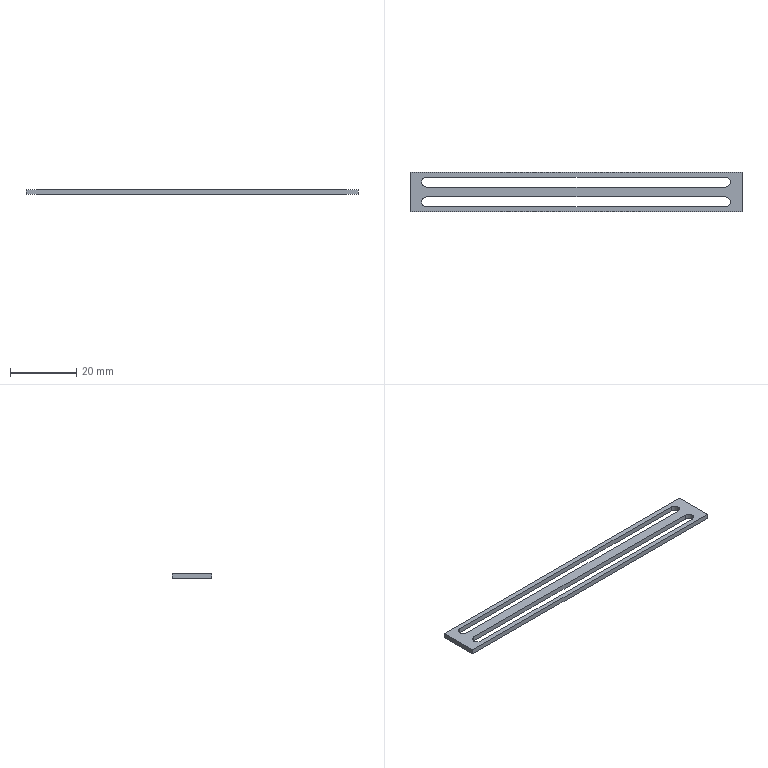Part | SolidWorks | features Extrusion 1 | 1 solid | 16 faces | box 100 x 12 x 1.5 mm | volume 968.794 mm3 | plane 10 | cylinder 6 | commonest cylinder face diameters 3 x6
STEP:
#1=CARTESIAN_POINT('',(-45.,-1.5,1.5));
#2=VERTEX_POINT('',#1);
#3=CARTESIAN_POINT('',(-46.5,-3.,1.5));
#4=VERTEX_POINT('',#3);
#5=CARTESIAN_POINT('',(-45.,-3.,1.5));
#6=DIRECTION('',(0.,0.,1.));
#7=DIRECTION('',(-1.,0.,0.));
#8=AXIS2_PLACEMENT_3D('',#5,#6,#7);
#9=CIRCLE('',#8,1.5);
#10=EDGE_CURVE('',#2,#4,#9,.T.);
#11=ORIENTED_EDGE('',*,*,#10,.T.);
#12=CARTESIAN_POINT('',(-46.5,-3.,0.));
#13=VERTEX_POINT('',#12);
#14=CARTESIAN_POINT('',(-46.5,-3.,1.5));
#15=DIRECTION('',(0.,0.,-1.));
#16=VECTOR('',#15,1000.);
#17=LINE('',#14,#16);
#18=EDGE_CURVE('',#4,#13,#17,.T.);
#19=ORIENTED_EDGE('',*,*,#18,.T.);
#20=CARTESIAN_POINT('',(-45.,-1.5,0.));
#21=VERTEX_POINT('',#20);
#22=CARTESIAN_POINT('',(-45.,-3.,0.));
#23=DIRECTION('',(0.,0.,1.));
#24=DIRECTION('',(-1.,0.,0.));
#25=AXIS2_PLACEMENT_3D('',#22,#23,#24);
#26=CIRCLE('',#25,1.5);
#27=EDGE_CURVE('',#21,#13,#26,.T.);
#28=ORIENTED_EDGE('',*,*,#27,.F.);
#29=CARTESIAN_POINT('',(-45.,-1.5,1.5));
#30=DIRECTION('',(0.,0.,-1.));
#31=VECTOR('',#30,1000.);
#32=LINE('',#29,#31);
#33=EDGE_CURVE('',#2,#21,#32,.T.);
#34=ORIENTED_EDGE('',*,*,#33,.F.);
#35=EDGE_LOOP('',(#11,#19,#28,#34));
#36=FACE_OUTER_BOUND('',#35,.T.);
#37=CARTESIAN_POINT('',(-45.,-3.,1.5));
#38=DIRECTION('',(0.,0.,-1.));
#39=DIRECTION('',(-1.,0.,0.));
#40=AXIS2_PLACEMENT_3D('',#37,#38,#39);
#41=CYLINDRICAL_SURFACE('',#40,1.5);
#42=ADVANCED_FACE('',(#36),#41,.F.);
#43=CARTESIAN_POINT('',(-45.,4.5,1.5));
#44=VERTEX_POINT('',#43);
#45=CARTESIAN_POINT('',(-46.5,3.,1.5));
#46=VERTEX_POINT('',#45);
#47=CARTESIAN_POINT('',(-45.,3.,1.5));
#48=DIRECTION('',(0.,0.,1.));
#49=DIRECTION('',(1.,0.,0.));
#50=AXIS2_PLACEMENT_3D('',#47,#48,#49);
#51=CIRCLE('',#50,1.5);
#52=EDGE_CURVE('',#44,#46,#51,.T.);
#53=ORIENTED_EDGE('',*,*,#52,.T.);
#54=CARTESIAN_POINT('',(-46.5,3.,0.));
#55=VERTEX_POINT('',#54);
#56=CARTESIAN_POINT('',(-46.5,3.,1.5));
#57=DIRECTION('',(0.,0.,-1.));
#58=VECTOR('',#57,1000.);
#59=LINE('',#56,#58);
#60=EDGE_CURVE('',#46,#55,#59,.T.);
#61=ORIENTED_EDGE('',*,*,#60,.T.);
#62=CARTESIAN_POINT('',(-45.,4.5,0.));
#63=VERTEX_POINT('',#62);
#64=CARTESIAN_POINT('',(-45.,3.,0.));
#65=DIRECTION('',(0.,0.,1.));
#66=DIRECTION('',(1.,0.,0.));
#67=AXIS2_PLACEMENT_3D('',#64,#65,#66);
#68=CIRCLE('',#67,1.5);
#69=EDGE_CURVE('',#63,#55,#68,.T.);
#70=ORIENTED_EDGE('',*,*,#69,.F.);
#71=CARTESIAN_POINT('',(-45.,4.5,1.5));
#72=DIRECTION('',(0.,0.,-1.));
#73=VECTOR('',#72,1000.);
#74=LINE('',#71,#73);
#75=EDGE_CURVE('',#44,#63,#74,.T.);
#76=ORIENTED_EDGE('',*,*,#75,.F.);
#77=EDGE_LOOP('',(#53,#61,#70,#76));
#78=FACE_OUTER_BOUND('',#77,.T.);
#79=CARTESIAN_POINT('',(-45.,3.,1.5));
#80=DIRECTION('',(0.,0.,-1.));
#81=DIRECTION('',(-1.,0.,0.));
#82=AXIS2_PLACEMENT_3D('',#79,#80,#81);
#83=CYLINDRICAL_SURFACE('',#82,1.5);
#84=ADVANCED_FACE('',(#78),#83,.F.);
#85=ORIENTED_EDGE('',*,*,#52,.F.);
#86=CARTESIAN_POINT('',(45.,4.5,1.5));
#87=VERTEX_POINT('',#86);
#88=CARTESIAN_POINT('',(-45.,4.5,1.5));
#89=DIRECTION('',(-1.,0.,0.));
#90=VECTOR('',#89,1000.);
#91=LINE('',#88,#90);
#92=EDGE_CURVE('',#87,#44,#91,.T.);
#93=ORIENTED_EDGE('',*,*,#92,.F.);
#94=CARTESIAN_POINT('',(45.,1.5,1.5));
#95=VERTEX_POINT('',#94);
#96=CARTESIAN_POINT('',(45.,3.,1.5));
#97=DIRECTION('',(0.,0.,1.));
#98=DIRECTION('',(1.,0.,0.));
#99=AXIS2_PLACEMENT_3D('',#96,#97,#98);
#100=CIRCLE('',#99,1.5);
#101=EDGE_CURVE('',#95,#87,#100,.T.);
#102=ORIENTED_EDGE('',*,*,#101,.F.);
#103=CARTESIAN_POINT('',(-45.,1.5,1.5));
#104=VERTEX_POINT('',#103);
#105=CARTESIAN_POINT('',(-45.,1.5,1.5));
#106=DIRECTION('',(1.,0.,0.));
#107=VECTOR('',#106,1000.);
#108=LINE('',#105,#107);
#109=EDGE_CURVE('',#104,#95,#108,.T.);
#110=ORIENTED_EDGE('',*,*,#109,.F.);
#111=CARTESIAN_POINT('',(-45.,3.,1.5));
#112=DIRECTION('',(0.,0.,1.));
#113=DIRECTION('',(1.,0.,0.));
#114=AXIS2_PLACEMENT_3D('',#111,#112,#113);
#115=CIRCLE('',#114,1.5);
#116=EDGE_CURVE('',#46,#104,#115,.T.);
#117=ORIENTED_EDGE('',*,*,#116,.F.);
#118=EDGE_LOOP('',(#85,#93,#102,#110,#117));
#119=FACE_BOUND('',#118,.T.);
#120=CARTESIAN_POINT('',(-50.,6.,1.5));
#121=VERTEX_POINT('',#120);
#122=CARTESIAN_POINT('',(-50.,-6.,1.5));
#123=VERTEX_POINT('',#122);
#124=CARTESIAN_POINT('',(-50.,6.,1.5));
#125=DIRECTION('',(0.,-1.,0.));
#126=VECTOR('',#125,1000.);
#127=LINE('',#124,#126);
#128=EDGE_CURVE('',#121,#123,#127,.T.);
#129=ORIENTED_EDGE('',*,*,#128,.T.);
#130=CARTESIAN_POINT('',(50.,-6.,1.5));
#131=VERTEX_POINT('',#130);
#132=CARTESIAN_POINT('',(50.,-6.,1.5));
#133=DIRECTION('',(1.,0.,0.));
#134=VECTOR('',#133,1000.);
#135=LINE('',#132,#134);
#136=EDGE_CURVE('',#123,#131,#135,.T.);
#137=ORIENTED_EDGE('',*,*,#136,.T.);
#138=CARTESIAN_POINT('',(50.,6.,1.5));
#139=VERTEX_POINT('',#138);
#140=CARTESIAN_POINT('',(50.,6.,1.5));
#141=DIRECTION('',(0.,1.,0.));
#142=VECTOR('',#141,1000.);
#143=LINE('',#140,#142);
#144=EDGE_CURVE('',#131,#139,#143,.T.);
#145=ORIENTED_EDGE('',*,*,#144,.T.);
#146=CARTESIAN_POINT('',(50.,6.,1.5));
#147=DIRECTION('',(-1.,0.,0.));
#148=VECTOR('',#147,1000.);
#149=LINE('',#146,#148);
#150=EDGE_CURVE('',#139,#121,#149,.T.);
#151=ORIENTED_EDGE('',*,*,#150,.T.);
#152=EDGE_LOOP('',(#129,#137,#145,#151));
#153=FACE_OUTER_BOUND('',#152,.T.);
#154=ORIENTED_EDGE('',*,*,#10,.F.);
#155=CARTESIAN_POINT('',(45.,-1.5,1.5));
#156=VERTEX_POINT('',#155);
#157=CARTESIAN_POINT('',(-45.,-1.5,1.5));
#158=DIRECTION('',(-1.,0.,0.));
#159=VECTOR('',#158,1000.);
#160=LINE('',#157,#159);
#161=EDGE_CURVE('',#156,#2,#160,.T.);
#162=ORIENTED_EDGE('',*,*,#161,.F.);
#163=CARTESIAN_POINT('',(45.,-4.5,1.5));
#164=VERTEX_POINT('',#163);
#165=CARTESIAN_POINT('',(45.,-3.,1.5));
#166=DIRECTION('',(0.,0.,1.));
#167=DIRECTION('',(-1.,0.,0.));
#168=AXIS2_PLACEMENT_3D('',#165,#166,#167);
#169=CIRCLE('',#168,1.5);
#170=EDGE_CURVE('',#164,#156,#169,.T.);
#171=ORIENTED_EDGE('',*,*,#170,.F.);
#172=CARTESIAN_POINT('',(-45.,-4.5,1.5));
#173=VERTEX_POINT('',#172);
#174=CARTESIAN_POINT('',(-45.,-4.5,1.5));
#175=DIRECTION('',(1.,0.,0.));
#176=VECTOR('',#175,1000.);
#177=LINE('',#174,#176);
#178=EDGE_CURVE('',#173,#164,#177,.T.);
#179=ORIENTED_EDGE('',*,*,#178,.F.);
#180=CARTESIAN_POINT('',(-45.,-3.,1.5));
#181=DIRECTION('',(0.,0.,1.));
#182=DIRECTION('',(-1.,0.,0.));
#183=AXIS2_PLACEMENT_3D('',#180,#181,#182);
#184=CIRCLE('',#183,1.5);
#185=EDGE_CURVE('',#4,#173,#184,.T.);
#186=ORIENTED_EDGE('',*,*,#185,.F.);
#187=EDGE_LOOP('',(#154,#162,#171,#179,#186));
#188=FACE_BOUND('',#187,.T.);
#189=CARTESIAN_POINT('',(0.,0.,1.5));
#190=DIRECTION('',(0.,0.,-1.));
#191=DIRECTION('',(-1.,0.,0.));
#192=AXIS2_PLACEMENT_3D('',#189,#190,#191);
#193=PLANE('',#192);
#194=ADVANCED_FACE('',(#119,#153,#188),#193,.F.);
#195=CARTESIAN_POINT('',(45.,4.5,0.));
#196=VERTEX_POINT('',#195);
#197=CARTESIAN_POINT('',(-45.,4.5,0.));
#198=DIRECTION('',(-1.,0.,0.));
#199=VECTOR('',#198,1000.);
#200=LINE('',#197,#199);
#201=EDGE_CURVE('',#196,#63,#200,.T.);
#202=ORIENTED_EDGE('',*,*,#201,.T.);
#203=ORIENTED_EDGE('',*,*,#69,.T.);
#204=CARTESIAN_POINT('',(-45.,1.5,0.));
#205=VERTEX_POINT('',#204);
#206=CARTESIAN_POINT('',(-45.,3.,0.));
#207=DIRECTION('',(0.,0.,1.));
#208=DIRECTION('',(1.,0.,0.));
#209=AXIS2_PLACEMENT_3D('',#206,#207,#208);
#210=CIRCLE('',#209,1.5);
#211=EDGE_CURVE('',#55,#205,#210,.T.);
#212=ORIENTED_EDGE('',*,*,#211,.T.);
#213=CARTESIAN_POINT('',(45.,1.5,0.));
#214=VERTEX_POINT('',#213);
#215=CARTESIAN_POINT('',(-45.,1.5,0.));
#216=DIRECTION('',(1.,0.,0.));
#217=VECTOR('',#216,1000.);
#218=LINE('',#215,#217);
#219=EDGE_CURVE('',#205,#214,#218,.T.);
#220=ORIENTED_EDGE('',*,*,#219,.T.);
#221=CARTESIAN_POINT('',(45.,3.,0.));
#222=DIRECTION('',(0.,0.,1.));
#223=DIRECTION('',(1.,0.,0.));
#224=AXIS2_PLACEMENT_3D('',#221,#222,#223);
#225=CIRCLE('',#224,1.5);
#226=EDGE_CURVE('',#214,#196,#225,.T.);
#227=ORIENTED_EDGE('',*,*,#226,.T.);
#228=EDGE_LOOP('',(#202,#203,#212,#220,#227));
#229=FACE_BOUND('',#228,.T.);
#230=CARTESIAN_POINT('',(-50.,6.,0.));
#231=VERTEX_POINT('',#230);
#232=CARTESIAN_POINT('',(-50.,-6.,0.));
#233=VERTEX_POINT('',#232);
#234=CARTESIAN_POINT('',(-50.,6.,0.));
#235=DIRECTION('',(0.,-1.,0.));
#236=VECTOR('',#235,1000.);
#237=LINE('',#234,#236);
#238=EDGE_CURVE('',#231,#233,#237,.T.);
#239=ORIENTED_EDGE('',*,*,#238,.F.);
#240=CARTESIAN_POINT('',(50.,6.,0.));
#241=VERTEX_POINT('',#240);
#242=CARTESIAN_POINT('',(50.,6.,0.));
#243=DIRECTION('',(-1.,0.,0.));
#244=VECTOR('',#243,1000.);
#245=LINE('',#242,#244);
#246=EDGE_CURVE('',#241,#231,#245,.T.);
#247=ORIENTED_EDGE('',*,*,#246,.F.);
#248=CARTESIAN_POINT('',(50.,-6.,0.));
#249=VERTEX_POINT('',#248);
#250=CARTESIAN_POINT('',(50.,6.,0.));
#251=DIRECTION('',(0.,1.,0.));
#252=VECTOR('',#251,1000.);
#253=LINE('',#250,#252);
#254=EDGE_CURVE('',#249,#241,#253,.T.);
#255=ORIENTED_EDGE('',*,*,#254,.F.);
#256=CARTESIAN_POINT('',(50.,-6.,0.));
#257=DIRECTION('',(1.,0.,0.));
#258=VECTOR('',#257,1000.);
#259=LINE('',#256,#258);
#260=EDGE_CURVE('',#233,#249,#259,.T.);
#261=ORIENTED_EDGE('',*,*,#260,.F.);
#262=EDGE_LOOP('',(#239,#247,#255,#261));
#263=FACE_OUTER_BOUND('',#262,.T.);
#264=CARTESIAN_POINT('',(45.,-1.5,0.));
#265=VERTEX_POINT('',#264);
#266=CARTESIAN_POINT('',(-45.,-1.5,0.));
#267=DIRECTION('',(-1.,0.,0.));
#268=VECTOR('',#267,1000.);
#269=LINE('',#266,#268);
#270=EDGE_CURVE('',#265,#21,#269,.T.);
#271=ORIENTED_EDGE('',*,*,#270,.T.);
#272=ORIENTED_EDGE('',*,*,#27,.T.);
#273=CARTESIAN_POINT('',(-45.,-4.5,0.));
#274=VERTEX_POINT('',#273);
#275=CARTESIAN_POINT('',(-45.,-3.,0.));
#276=DIRECTION('',(0.,0.,1.));
#277=DIRECTION('',(-1.,0.,0.));
#278=AXIS2_PLACEMENT_3D('',#275,#276,#277);
#279=CIRCLE('',#278,1.5);
#280=EDGE_CURVE('',#13,#274,#279,.T.);
#281=ORIENTED_EDGE('',*,*,#280,.T.);
#282=CARTESIAN_POINT('',(45.,-4.5,0.));
#283=VERTEX_POINT('',#282);
#284=CARTESIAN_POINT('',(-45.,-4.5,0.));
#285=DIRECTION('',(1.,0.,0.));
#286=VECTOR('',#285,1000.);
#287=LINE('',#284,#286);
#288=EDGE_CURVE('',#274,#283,#287,.T.);
#289=ORIENTED_EDGE('',*,*,#288,.T.);
#290=CARTESIAN_POINT('',(45.,-3.,0.));
#291=DIRECTION('',(0.,0.,1.));
#292=DIRECTION('',(-1.,0.,0.));
#293=AXIS2_PLACEMENT_3D('',#290,#291,#292);
#294=CIRCLE('',#293,1.5);
#295=EDGE_CURVE('',#283,#265,#294,.T.);
#296=ORIENTED_EDGE('',*,*,#295,.T.);
#297=EDGE_LOOP('',(#271,#272,#281,#289,#296));
#298=FACE_BOUND('',#297,.T.);
#299=CARTESIAN_POINT('',(0.,0.,0.));
#300=DIRECTION('',(0.,0.,-1.));
#301=DIRECTION('',(-1.,0.,0.));
#302=AXIS2_PLACEMENT_3D('',#299,#300,#301);
#303=PLANE('',#302);
#304=ADVANCED_FACE('',(#229,#263,#298),#303,.T.);
#305=ORIENTED_EDGE('',*,*,#238,.T.);
#306=CARTESIAN_POINT('',(-50.,-6.,1.5));
#307=DIRECTION('',(0.,0.,-1.));
#308=VECTOR('',#307,1000.);
#309=LINE('',#306,#308);
#310=EDGE_CURVE('',#123,#233,#309,.T.);
#311=ORIENTED_EDGE('',*,*,#310,.F.);
#312=ORIENTED_EDGE('',*,*,#128,.F.);
#313=CARTESIAN_POINT('',(-50.,6.,1.5));
#314=DIRECTION('',(0.,0.,-1.));
#315=VECTOR('',#314,1000.);
#316=LINE('',#313,#315);
#317=EDGE_CURVE('',#121,#231,#316,.T.);
#318=ORIENTED_EDGE('',*,*,#317,.T.);
#319=EDGE_LOOP('',(#305,#311,#312,#318));
#320=FACE_OUTER_BOUND('',#319,.T.);
#321=CARTESIAN_POINT('',(-50.,6.,1.5));
#322=DIRECTION('',(1.,0.,0.));
#323=DIRECTION('',(0.,0.,-1.));
#324=AXIS2_PLACEMENT_3D('',#321,#322,#323);
#325=PLANE('',#324);
#326=ADVANCED_FACE('',(#320),#325,.F.);
#327=ORIENTED_EDGE('',*,*,#260,.T.);
#328=CARTESIAN_POINT('',(50.,-6.,1.5));
#329=DIRECTION('',(0.,0.,-1.));
#330=VECTOR('',#329,1000.);
#331=LINE('',#328,#330);
#332=EDGE_CURVE('',#131,#249,#331,.T.);
#333=ORIENTED_EDGE('',*,*,#332,.F.);
#334=ORIENTED_EDGE('',*,*,#136,.F.);
#335=ORIENTED_EDGE('',*,*,#310,.T.);
#336=EDGE_LOOP('',(#327,#333,#334,#335));
#337=FACE_OUTER_BOUND('',#336,.T.);
#338=CARTESIAN_POINT('',(50.,-6.,1.5));
#339=DIRECTION('',(0.,1.,0.));
#340=DIRECTION('',(-1.,0.,0.));
#341=AXIS2_PLACEMENT_3D('',#338,#339,#340);
#342=PLANE('',#341);
#343=ADVANCED_FACE('',(#337),#342,.F.);
#344=ORIENTED_EDGE('',*,*,#254,.T.);
#345=CARTESIAN_POINT('',(50.,6.,1.5));
#346=DIRECTION('',(0.,0.,-1.));
#347=VECTOR('',#346,1000.);
#348=LINE('',#345,#347);
#349=EDGE_CURVE('',#139,#241,#348,.T.);
#350=ORIENTED_EDGE('',*,*,#349,.F.);
#351=ORIENTED_EDGE('',*,*,#144,.F.);
#352=ORIENTED_EDGE('',*,*,#332,.T.);
#353=EDGE_LOOP('',(#344,#350,#351,#352));
#354=FACE_OUTER_BOUND('',#353,.T.);
#355=CARTESIAN_POINT('',(50.,6.,1.5));
#356=DIRECTION('',(-1.,0.,0.));
#357=DIRECTION('',(0.,0.,1.));
#358=AXIS2_PLACEMENT_3D('',#355,#356,#357);
#359=PLANE('',#358);
#360=ADVANCED_FACE('',(#354),#359,.F.);
#361=ORIENTED_EDGE('',*,*,#246,.T.);
#362=ORIENTED_EDGE('',*,*,#317,.F.);
#363=ORIENTED_EDGE('',*,*,#150,.F.);
#364=ORIENTED_EDGE('',*,*,#349,.T.);
#365=EDGE_LOOP('',(#361,#362,#363,#364));
#366=FACE_OUTER_BOUND('',#365,.T.);
#367=CARTESIAN_POINT('',(50.,6.,1.5));
#368=DIRECTION('',(0.,-1.,0.));
#369=DIRECTION('',(1.,0.,0.));
#370=AXIS2_PLACEMENT_3D('',#367,#368,#369);
#371=PLANE('',#370);
#372=ADVANCED_FACE('',(#366),#371,.F.);
#373=ORIENTED_EDGE('',*,*,#60,.F.);
#374=ORIENTED_EDGE('',*,*,#116,.T.);
#375=CARTESIAN_POINT('',(-45.,1.5,1.5));
#376=DIRECTION('',(0.,0.,-1.));
#377=VECTOR('',#376,1000.);
#378=LINE('',#375,#377);
#379=EDGE_CURVE('',#104,#205,#378,.T.);
#380=ORIENTED_EDGE('',*,*,#379,.T.);
#381=ORIENTED_EDGE('',*,*,#211,.F.);
#382=EDGE_LOOP('',(#373,#374,#380,#381));
#383=FACE_OUTER_BOUND('',#382,.T.);
#384=CARTESIAN_POINT('',(-45.,3.,1.5));
#385=DIRECTION('',(0.,0.,-1.));
#386=DIRECTION('',(-1.,0.,0.));
#387=AXIS2_PLACEMENT_3D('',#384,#385,#386);
#388=CYLINDRICAL_SURFACE('',#387,1.5);
#389=ADVANCED_FACE('',(#383),#388,.F.);
#390=ORIENTED_EDGE('',*,*,#219,.F.);
#391=ORIENTED_EDGE('',*,*,#379,.F.);
#392=ORIENTED_EDGE('',*,*,#109,.T.);
#393=CARTESIAN_POINT('',(45.,1.5,1.5));
#394=DIRECTION('',(0.,0.,-1.));
#395=VECTOR('',#394,1000.);
#396=LINE('',#393,#395);
#397=EDGE_CURVE('',#95,#214,#396,.T.);
#398=ORIENTED_EDGE('',*,*,#397,.T.);
#399=EDGE_LOOP('',(#390,#391,#392,#398));
#400=FACE_OUTER_BOUND('',#399,.T.);
#401=CARTESIAN_POINT('',(-45.,1.5,1.5));
#402=DIRECTION('',(0.,1.,0.));
#403=DIRECTION('',(-1.,0.,0.));
#404=AXIS2_PLACEMENT_3D('',#401,#402,#403);
#405=PLANE('',#404);
#406=ADVANCED_FACE('',(#400),#405,.T.);
#407=ORIENTED_EDGE('',*,*,#226,.F.);
#408=ORIENTED_EDGE('',*,*,#397,.F.);
#409=ORIENTED_EDGE('',*,*,#101,.T.);
#410=CARTESIAN_POINT('',(45.,4.5,1.5));
#411=DIRECTION('',(0.,0.,-1.));
#412=VECTOR('',#411,1000.);
#413=LINE('',#410,#412);
#414=EDGE_CURVE('',#87,#196,#413,.T.);
#415=ORIENTED_EDGE('',*,*,#414,.T.);
#416=EDGE_LOOP('',(#407,#408,#409,#415));
#417=FACE_OUTER_BOUND('',#416,.T.);
#418=CARTESIAN_POINT('',(45.,3.,1.5));
#419=DIRECTION('',(0.,0.,-1.));
#420=DIRECTION('',(-1.,0.,0.));
#421=AXIS2_PLACEMENT_3D('',#418,#419,#420);
#422=CYLINDRICAL_SURFACE('',#421,1.5);
#423=ADVANCED_FACE('',(#417),#422,.F.);
#424=ORIENTED_EDGE('',*,*,#201,.F.);
#425=ORIENTED_EDGE('',*,*,#414,.F.);
#426=ORIENTED_EDGE('',*,*,#92,.T.);
#427=ORIENTED_EDGE('',*,*,#75,.T.);
#428=EDGE_LOOP('',(#424,#425,#426,#427));
#429=FACE_OUTER_BOUND('',#428,.T.);
#430=CARTESIAN_POINT('',(-45.,4.5,1.5));
#431=DIRECTION('',(0.,-1.,0.));
#432=DIRECTION('',(1.,0.,0.));
#433=AXIS2_PLACEMENT_3D('',#430,#431,#432);
#434=PLANE('',#433);
#435=ADVANCED_FACE('',(#429),#434,.T.);
#436=ORIENTED_EDGE('',*,*,#18,.F.);
#437=ORIENTED_EDGE('',*,*,#185,.T.);
#438=CARTESIAN_POINT('',(-45.,-4.5,1.5));
#439=DIRECTION('',(0.,0.,-1.));
#440=VECTOR('',#439,1000.);
#441=LINE('',#438,#440);
#442=EDGE_CURVE('',#173,#274,#441,.T.);
#443=ORIENTED_EDGE('',*,*,#442,.T.);
#444=ORIENTED_EDGE('',*,*,#280,.F.);
#445=EDGE_LOOP('',(#436,#437,#443,#444));
#446=FACE_OUTER_BOUND('',#445,.T.);
#447=CARTESIAN_POINT('',(-45.,-3.,1.5));
#448=DIRECTION('',(0.,0.,-1.));
#449=DIRECTION('',(-1.,0.,0.));
#450=AXIS2_PLACEMENT_3D('',#447,#448,#449);
#451=CYLINDRICAL_SURFACE('',#450,1.5);
#452=ADVANCED_FACE('',(#446),#451,.F.);
#453=ORIENTED_EDGE('',*,*,#288,.F.);
#454=ORIENTED_EDGE('',*,*,#442,.F.);
#455=ORIENTED_EDGE('',*,*,#178,.T.);
#456=CARTESIAN_POINT('',(45.,-4.5,1.5));
#457=DIRECTION('',(0.,0.,-1.));
#458=VECTOR('',#457,1000.);
#459=LINE('',#456,#458);
#460=EDGE_CURVE('',#164,#283,#459,.T.);
#461=ORIENTED_EDGE('',*,*,#460,.T.);
#462=EDGE_LOOP('',(#453,#454,#455,#461));
#463=FACE_OUTER_BOUND('',#462,.T.);
#464=CARTESIAN_POINT('',(-45.,-4.5,1.5));
#465=DIRECTION('',(0.,1.,0.));
#466=DIRECTION('',(-1.,0.,0.));
#467=AXIS2_PLACEMENT_3D('',#464,#465,#466);
#468=PLANE('',#467);
#469=ADVANCED_FACE('',(#463),#468,.T.);
#470=ORIENTED_EDGE('',*,*,#295,.F.);
#471=ORIENTED_EDGE('',*,*,#460,.F.);
#472=ORIENTED_EDGE('',*,*,#170,.T.);
#473=CARTESIAN_POINT('',(45.,-1.5,1.5));
#474=DIRECTION('',(0.,0.,-1.));
#475=VECTOR('',#474,1000.);
#476=LINE('',#473,#475);
#477=EDGE_CURVE('',#156,#265,#476,.T.);
#478=ORIENTED_EDGE('',*,*,#477,.T.);
#479=EDGE_LOOP('',(#470,#471,#472,#478));
#480=FACE_OUTER_BOUND('',#479,.T.);
#481=CARTESIAN_POINT('',(45.,-3.,1.5));
#482=DIRECTION('',(0.,0.,-1.));
#483=DIRECTION('',(-1.,0.,0.));
#484=AXIS2_PLACEMENT_3D('',#481,#482,#483);
#485=CYLINDRICAL_SURFACE('',#484,1.5);
#486=ADVANCED_FACE('',(#480),#485,.F.);
#487=ORIENTED_EDGE('',*,*,#270,.F.);
#488=ORIENTED_EDGE('',*,*,#477,.F.);
#489=ORIENTED_EDGE('',*,*,#161,.T.);
#490=ORIENTED_EDGE('',*,*,#33,.T.);
#491=EDGE_LOOP('',(#487,#488,#489,#490));
#492=FACE_OUTER_BOUND('',#491,.T.);
#493=CARTESIAN_POINT('',(-45.,-1.5,1.5));
#494=DIRECTION('',(0.,-1.,0.));
#495=DIRECTION('',(1.,0.,0.));
#496=AXIS2_PLACEMENT_3D('',#493,#494,#495);
#497=PLANE('',#496);
#498=ADVANCED_FACE('',(#492),#497,.T.);
#499=CLOSED_SHELL('',(#42,#84,#194,#304,#326,#343,#360,#372,#389,#406,#423,#435,#452,#469,#486,#498));
#500=MANIFOLD_SOLID_BREP('',#499);
#501=CARTESIAN_POINT('',(0.,0.,0.));
#502=DIRECTION('',(0.,0.,1.));
#503=DIRECTION('',(1.,0.,0.));
#504=AXIS2_PLACEMENT_3D('',#501,#502,#503);
#505=(LENGTH_UNIT()NAMED_UNIT(*)SI_UNIT(.MILLI.,.METRE.));
#506=UNCERTAINTY_MEASURE_WITH_UNIT(LENGTH_MEASURE(0.00001),#505,'','');
#507=(NAMED_UNIT(*)PLANE_ANGLE_UNIT()SI_UNIT($,.RADIAN.));
#508=(NAMED_UNIT(*)SI_UNIT($,.STERADIAN.)SOLID_ANGLE_UNIT());
#509=(GEOMETRIC_REPRESENTATION_CONTEXT(3)GLOBAL_UNCERTAINTY_ASSIGNED_CONTEXT((#506))GLOBAL_UNIT_ASSIGNED_CONTEXT((#505,#507,#508))REPRESENTATION_CONTEXT('',''));
#510=ADVANCED_BREP_SHAPE_REPRESENTATION('',(#500,#504),#509);